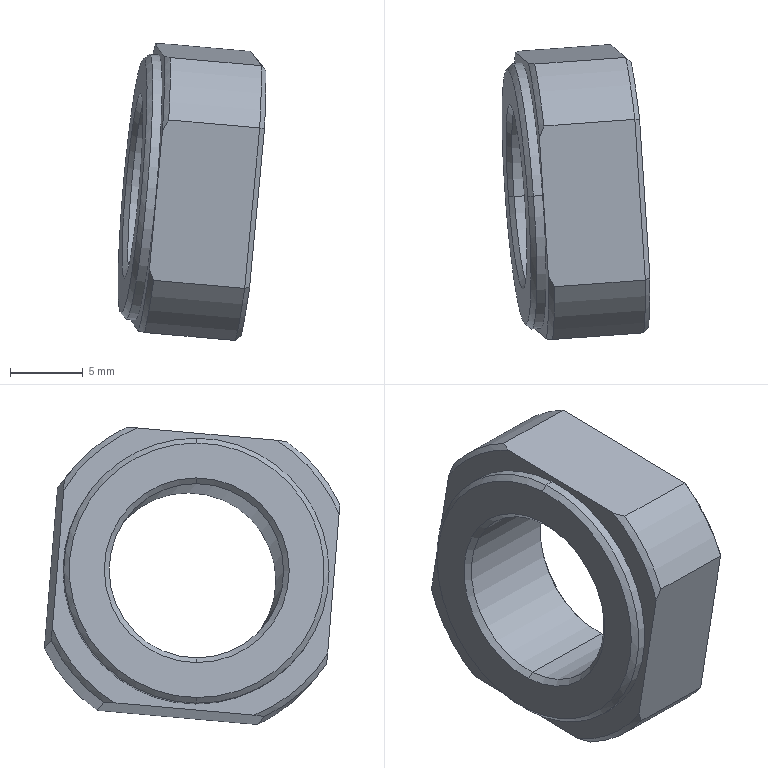Part | STEP file | 1 solid | 33 faces | box 10.153 x 20.245 x 20.375 mm | volume 1688 mm3 | cone 14 | plane 11 | cylinder 8 | commonest cylinder face diameters 22 x4 12 x2 18.246 x2